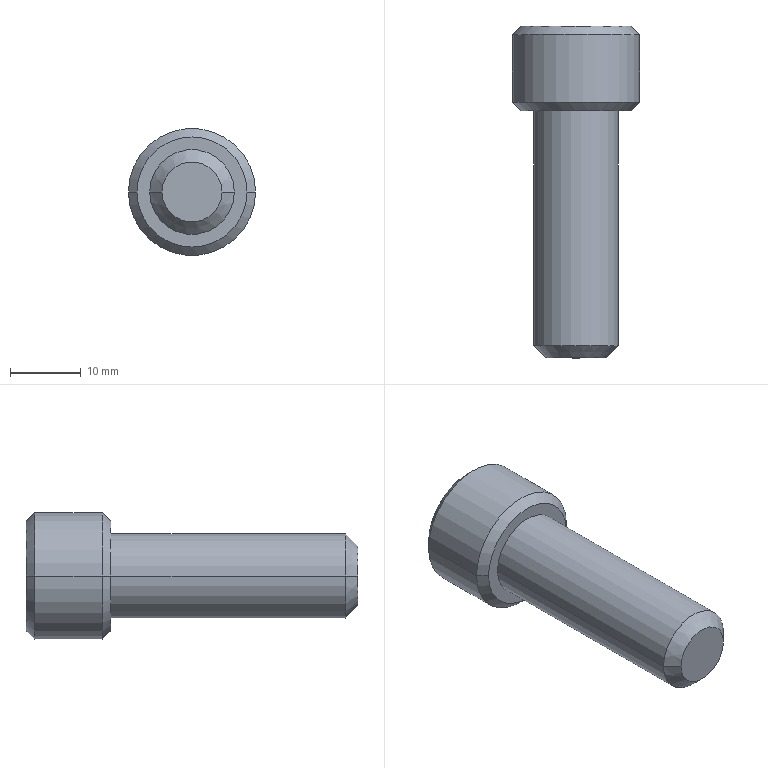Part | STEP file | BB62-M12-35L | 1 solid | 27 faces | box 18 x 47 x 18 mm | volume 6260 mm3 | plane 15 | cone 8 | cylinder 4 | commonest cylinder face diameters 12 x2 18 x2